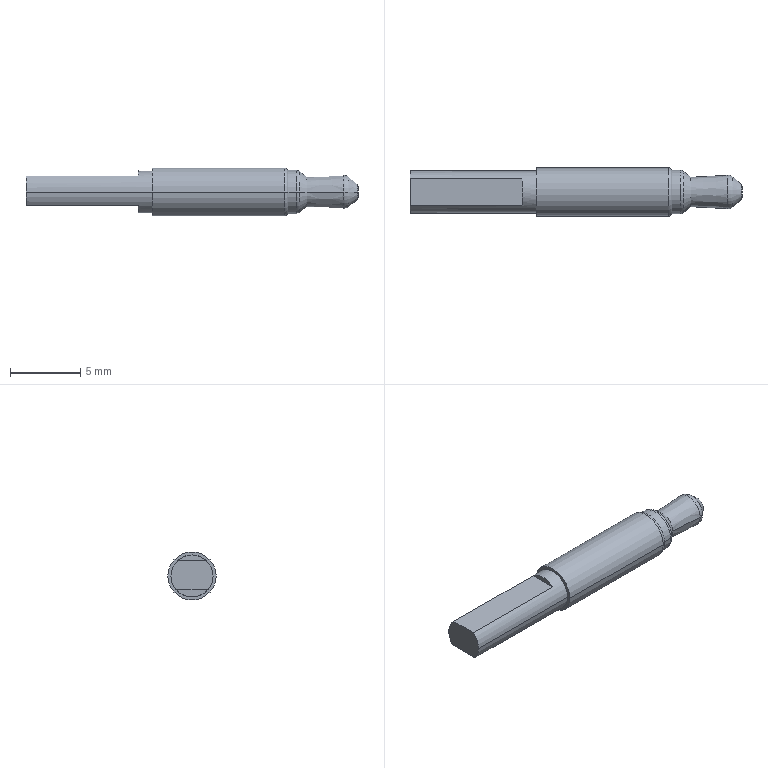Part | NX | 1 solid | 27 faces | box 23.7 x 3.45 x 3.45 mm | volume 165.514 mm3 | torus 8 | plane 7 | cylinder 6 | cone 6 | commonest cylinder face diameters 3 x2 3.1 x2 3.45 x2
STEP:
#1=CARTESIAN_POINT('',(12.641,-1.55,0.));
#2=VERTEX_POINT('',#1);
#3=CARTESIAN_POINT('',(12.641,1.55,0.));
#4=VERTEX_POINT('',#3);
#5=CARTESIAN_POINT('',(12.641,0.,0.));
#6=DIRECTION('',(1.,0.,0.));
#7=DIRECTION('',(0.,-1.,0.));
#8=AXIS2_PLACEMENT_3D('',#5,#6,#7);
#9=CIRCLE('',#8,1.55);
#10=EDGE_CURVE('',#2,#4,#9,.T.);
#11=ORIENTED_EDGE('',*,*,#10,.F.);
#12=CARTESIAN_POINT('',(12.,-1.55,0.));
#13=VERTEX_POINT('',#12);
#14=CARTESIAN_POINT('',(-0.85,-1.55,0.));
#15=DIRECTION('',(1.,0.,0.));
#16=VECTOR('',#15,1000.);
#17=LINE('',#14,#16);
#18=EDGE_CURVE('',#2,#13,#17,.F.);
#19=ORIENTED_EDGE('',*,*,#18,.T.);
#20=CARTESIAN_POINT('',(12.,1.55,0.));
#21=VERTEX_POINT('',#20);
#22=CARTESIAN_POINT('',(12.,0.,0.));
#23=DIRECTION('',(1.,0.,0.));
#24=DIRECTION('',(0.,1.,0.));
#25=AXIS2_PLACEMENT_3D('',#22,#23,#24);
#26=CIRCLE('',#25,1.55);
#27=EDGE_CURVE('',#13,#21,#26,.T.);
#28=ORIENTED_EDGE('',*,*,#27,.T.);
#29=CARTESIAN_POINT('',(-0.85,1.55,0.));
#30=DIRECTION('',(1.,0.,0.));
#31=VECTOR('',#30,1000.);
#32=LINE('',#29,#31);
#33=EDGE_CURVE('',#4,#21,#32,.F.);
#34=ORIENTED_EDGE('',*,*,#33,.F.);
#35=EDGE_LOOP('',(#11,#19,#28,#34));
#36=FACE_BOUND('',#35,.T.);
#37=CARTESIAN_POINT('',(-0.85,0.,0.));
#38=DIRECTION('',(1.,0.,0.));
#39=DIRECTION('',(0.,-1.,0.));
#40=AXIS2_PLACEMENT_3D('',#37,#38,#39);
#41=CYLINDRICAL_SURFACE('',#40,1.55);
#42=ADVANCED_FACE('',(#36),#41,.T.);
#43=CARTESIAN_POINT('',(13.35,1.05,0.));
#44=VERTEX_POINT('',#43);
#45=CARTESIAN_POINT('',(13.35,-1.05,0.));
#46=VERTEX_POINT('',#45);
#47=CARTESIAN_POINT('',(13.35,0.,0.));
#48=DIRECTION('',(1.,0.,0.));
#49=DIRECTION('',(0.,0.,-1.));
#50=AXIS2_PLACEMENT_3D('',#47,#48,#49);
#51=CIRCLE('',#50,1.05);
#52=EDGE_CURVE('',#44,#46,#51,.T.);
#53=ORIENTED_EDGE('',*,*,#52,.F.);
#54=CARTESIAN_POINT('',(12.833,1.48,0.));
#55=VERTEX_POINT('',#54);
#56=CARTESIAN_POINT('',(13.05,1.3,0.));
#57=DIRECTION('',(-0.7682,0.6402,0.));
#58=VECTOR('',#57,1000.);
#59=LINE('',#56,#58);
#60=EDGE_CURVE('',#44,#55,#59,.T.);
#61=ORIENTED_EDGE('',*,*,#60,.T.);
#62=CARTESIAN_POINT('',(12.833,-1.48,0.));
#63=VERTEX_POINT('',#62);
#64=CARTESIAN_POINT('',(12.833,0.,0.));
#65=DIRECTION('',(1.,0.,0.));
#66=DIRECTION('',(0.,-1.,0.));
#67=AXIS2_PLACEMENT_3D('',#64,#65,#66);
#68=CIRCLE('',#67,1.48);
#69=EDGE_CURVE('',#55,#63,#68,.T.);
#70=ORIENTED_EDGE('',*,*,#69,.T.);
#71=CARTESIAN_POINT('',(13.05,-1.3,0.));
#72=DIRECTION('',(-0.7682,-0.6402,0.));
#73=VECTOR('',#72,1000.);
#74=LINE('',#71,#73);
#75=EDGE_CURVE('',#46,#63,#74,.T.);
#76=ORIENTED_EDGE('',*,*,#75,.F.);
#77=EDGE_LOOP('',(#53,#61,#70,#76));
#78=FACE_BOUND('',#77,.T.);
#79=CARTESIAN_POINT('',(13.05,0.,0.));
#80=DIRECTION('',(-1.,0.,0.));
#81=DIRECTION('',(0.,1.,0.));
#82=AXIS2_PLACEMENT_3D('',#79,#80,#81);
#83=CONICAL_SURFACE('',#82,1.3,0.6947);
#84=ADVANCED_FACE('',(#78),#83,.T.);
#85=CARTESIAN_POINT('',(16.932,-0.5598,0.));
#86=VERTEX_POINT('',#85);
#87=CARTESIAN_POINT('',(16.932,0.5598,0.));
#88=VERTEX_POINT('',#87);
#89=CARTESIAN_POINT('',(16.932,0.,0.));
#90=DIRECTION('',(-1.,0.,0.));
#91=DIRECTION('',(0.,-1.,0.));
#92=AXIS2_PLACEMENT_3D('',#89,#90,#91);
#93=CIRCLE('',#92,0.5598);
#94=EDGE_CURVE('',#86,#88,#93,.T.);
#95=ORIENTED_EDGE('',*,*,#94,.T.);
#96=CARTESIAN_POINT('',(16.353,1.066,0.));
#97=VERTEX_POINT('',#96);
#98=CARTESIAN_POINT('',(16.596,0.8531,0.));
#99=DIRECTION('',(-0.7526,0.6585,0.));
#100=VECTOR('',#99,1000.);
#101=LINE('',#98,#100);
#102=EDGE_CURVE('',#88,#97,#101,.T.);
#103=ORIENTED_EDGE('',*,*,#102,.T.);
#104=CARTESIAN_POINT('',(16.353,-1.066,0.));
#105=VERTEX_POINT('',#104);
#106=CARTESIAN_POINT('',(16.353,0.,0.));
#107=DIRECTION('',(-1.,0.,0.));
#108=DIRECTION('',(0.,1.,0.));
#109=AXIS2_PLACEMENT_3D('',#106,#107,#108);
#110=CIRCLE('',#109,1.066);
#111=EDGE_CURVE('',#105,#97,#110,.T.);
#112=ORIENTED_EDGE('',*,*,#111,.F.);
#113=CARTESIAN_POINT('',(16.596,-0.8531,0.));
#114=DIRECTION('',(-0.7526,-0.6585,0.));
#115=VECTOR('',#114,1000.);
#116=LINE('',#113,#115);
#117=EDGE_CURVE('',#86,#105,#116,.T.);
#118=ORIENTED_EDGE('',*,*,#117,.F.);
#119=EDGE_LOOP('',(#95,#103,#112,#118));
#120=FACE_BOUND('',#119,.T.);
#121=CARTESIAN_POINT('',(16.596,0.,0.));
#122=DIRECTION('',(-1.,0.,0.));
#123=DIRECTION('',(0.,1.,0.));
#124=AXIS2_PLACEMENT_3D('',#121,#122,#123);
#125=CONICAL_SURFACE('',#124,0.8531,0.7188);
#126=ADVANCED_FACE('',(#120),#125,.T.);
#127=CARTESIAN_POINT('',(17.,-0.4092,0.));
#128=VERTEX_POINT('',#127);
#129=CARTESIAN_POINT('',(17.,0.4092,0.));
#130=VERTEX_POINT('',#129);
#131=CARTESIAN_POINT('',(17.,0.,0.));
#132=DIRECTION('',(1.,0.,0.));
#133=DIRECTION('',(0.,-1.,0.));
#134=AXIS2_PLACEMENT_3D('',#131,#132,#133);
#135=CIRCLE('',#134,0.4092);
#136=EDGE_CURVE('',#128,#130,#135,.T.);
#137=ORIENTED_EDGE('',*,*,#136,.T.);
#138=CARTESIAN_POINT('',(17.,0.,0.));
#139=DIRECTION('',(1.,0.,0.));
#140=DIRECTION('',(0.,-1.,0.));
#141=AXIS2_PLACEMENT_3D('',#138,#139,#140);
#142=CIRCLE('',#141,0.4092);
#143=EDGE_CURVE('',#130,#128,#142,.T.);
#144=ORIENTED_EDGE('',*,*,#143,.T.);
#145=EDGE_LOOP('',(#137,#144));
#146=FACE_BOUND('',#145,.T.);
#147=CARTESIAN_POINT('',(17.,0.,0.));
#148=DIRECTION('',(1.,0.,0.));
#149=DIRECTION('',(0.,1.,0.));
#150=AXIS2_PLACEMENT_3D('',#147,#148,#149);
#151=PLANE('',#150);
#152=ADVANCED_FACE('',(#146),#151,.T.);
#153=CARTESIAN_POINT('',(11.727,-1.725,0.));
#154=VERTEX_POINT('',#153);
#155=CARTESIAN_POINT('',(11.727,1.725,0.));
#156=VERTEX_POINT('',#155);
#157=CARTESIAN_POINT('',(11.727,0.,0.));
#158=DIRECTION('',(1.,0.,0.));
#159=DIRECTION('',(0.,-1.,0.));
#160=AXIS2_PLACEMENT_3D('',#157,#158,#159);
#161=CIRCLE('',#160,1.725);
#162=EDGE_CURVE('',#154,#156,#161,.T.);
#163=ORIENTED_EDGE('',*,*,#162,.T.);
#164=CARTESIAN_POINT('',(11.727,1.425,0.));
#165=DIRECTION('',(0.,0.,1.));
#166=DIRECTION('',(-1.,0.,0.));
#167=AXIS2_PLACEMENT_3D('',#164,#165,#166);
#168=CIRCLE('',#167,0.3);
#169=EDGE_CURVE('',#21,#156,#168,.T.);
#170=ORIENTED_EDGE('',*,*,#169,.F.);
#171=ORIENTED_EDGE('',*,*,#27,.F.);
#172=CARTESIAN_POINT('',(11.727,-1.425,0.));
#173=DIRECTION('',(0.,0.,-1.));
#174=DIRECTION('',(-1.,0.,0.));
#175=AXIS2_PLACEMENT_3D('',#172,#173,#174);
#176=CIRCLE('',#175,0.3);
#177=EDGE_CURVE('',#13,#154,#176,.T.);
#178=ORIENTED_EDGE('',*,*,#177,.T.);
#179=EDGE_LOOP('',(#163,#170,#171,#178));
#180=FACE_BOUND('',#179,.T.);
#181=CARTESIAN_POINT('',(11.727,0.,0.));
#182=DIRECTION('',(1.,0.,0.));
#183=DIRECTION('',(0.,-1.,0.));
#184=AXIS2_PLACEMENT_3D('',#181,#182,#183);
#185=TOROIDAL_SURFACE('',#184,1.425,0.3);
#186=ADVANCED_FACE('',(#180),#185,.T.);
#187=CARTESIAN_POINT('',(15.997,-1.189,0.));
#188=VERTEX_POINT('',#187);
#189=CARTESIAN_POINT('',(15.997,1.189,0.));
#190=VERTEX_POINT('',#189);
#191=CARTESIAN_POINT('',(15.997,0.,0.));
#192=DIRECTION('',(-1.,0.,0.));
#193=DIRECTION('',(0.,1.,0.));
#194=AXIS2_PLACEMENT_3D('',#191,#192,#193);
#195=CIRCLE('',#194,1.189);
#196=EDGE_CURVE('',#188,#190,#195,.T.);
#197=ORIENTED_EDGE('',*,*,#196,.F.);
#198=CARTESIAN_POINT('',(16.024,-0.69,0.));
#199=DIRECTION('',(0.,0.,1.));
#200=DIRECTION('',(-1.,0.,0.));
#201=AXIS2_PLACEMENT_3D('',#198,#199,#200);
#202=CIRCLE('',#201,0.5);
#203=EDGE_CURVE('',#188,#105,#202,.T.);
#204=ORIENTED_EDGE('',*,*,#203,.T.);
#205=ORIENTED_EDGE('',*,*,#111,.T.);
#206=CARTESIAN_POINT('',(16.024,0.69,0.));
#207=DIRECTION('',(0.,0.,-1.));
#208=DIRECTION('',(-1.,0.,0.));
#209=AXIS2_PLACEMENT_3D('',#206,#207,#208);
#210=CIRCLE('',#209,0.5);
#211=EDGE_CURVE('',#190,#97,#210,.T.);
#212=ORIENTED_EDGE('',*,*,#211,.F.);
#213=EDGE_LOOP('',(#197,#204,#205,#212));
#214=FACE_BOUND('',#213,.T.);
#215=CARTESIAN_POINT('',(16.024,0.,0.));
#216=DIRECTION('',(-1.,0.,0.));
#217=DIRECTION('',(0.,1.,0.));
#218=AXIS2_PLACEMENT_3D('',#215,#216,#217);
#219=TOROIDAL_SURFACE('',#218,0.69,0.5);
#220=ADVANCED_FACE('',(#214),#219,.T.);
#221=CARTESIAN_POINT('',(2.3,1.725,0.));
#222=VERTEX_POINT('',#221);
#223=CARTESIAN_POINT('',(2.3,-1.725,0.));
#224=VERTEX_POINT('',#223);
#225=CARTESIAN_POINT('',(2.3,0.,0.));
#226=DIRECTION('',(1.,0.,0.));
#227=DIRECTION('',(0.,-1.,0.));
#228=AXIS2_PLACEMENT_3D('',#225,#226,#227);
#229=CIRCLE('',#228,1.725);
#230=EDGE_CURVE('',#222,#224,#229,.T.);
#231=ORIENTED_EDGE('',*,*,#230,.T.);
#232=CARTESIAN_POINT('',(0.,-1.725,0.));
#233=DIRECTION('',(1.,0.,0.));
#234=VECTOR('',#233,1000.);
#235=LINE('',#232,#234);
#236=EDGE_CURVE('',#154,#224,#235,.F.);
#237=ORIENTED_EDGE('',*,*,#236,.F.);
#238=CARTESIAN_POINT('',(11.727,0.,0.));
#239=DIRECTION('',(1.,0.,0.));
#240=DIRECTION('',(0.,-1.,0.));
#241=AXIS2_PLACEMENT_3D('',#238,#239,#240);
#242=CIRCLE('',#241,1.725);
#243=EDGE_CURVE('',#156,#154,#242,.T.);
#244=ORIENTED_EDGE('',*,*,#243,.F.);
#245=CARTESIAN_POINT('',(0.,1.725,0.));
#246=DIRECTION('',(1.,0.,0.));
#247=VECTOR('',#246,1000.);
#248=LINE('',#245,#247);
#249=EDGE_CURVE('',#156,#222,#248,.F.);
#250=ORIENTED_EDGE('',*,*,#249,.T.);
#251=EDGE_LOOP('',(#231,#237,#244,#250));
#252=FACE_BOUND('',#251,.T.);
#253=CARTESIAN_POINT('',(0.,0.,0.));
#254=DIRECTION('',(1.,0.,0.));
#255=DIRECTION('',(0.,-1.,0.));
#256=AXIS2_PLACEMENT_3D('',#253,#254,#255);
#257=CYLINDRICAL_SURFACE('',#256,1.725);
#258=ADVANCED_FACE('',(#252),#257,.T.);
#259=ORIENTED_EDGE('',*,*,#52,.T.);
#260=CARTESIAN_POINT('',(14.734,-1.123,0.));
#261=DIRECTION('',(0.9986,-0.05256,0.));
#262=VECTOR('',#261,1000.);
#263=LINE('',#260,#262);
#264=EDGE_CURVE('',#188,#46,#263,.F.);
#265=ORIENTED_EDGE('',*,*,#264,.F.);
#266=ORIENTED_EDGE('',*,*,#196,.T.);
#267=CARTESIAN_POINT('',(14.734,1.123,0.));
#268=DIRECTION('',(0.9986,0.05256,0.));
#269=VECTOR('',#268,1000.);
#270=LINE('',#267,#269);
#271=EDGE_CURVE('',#190,#44,#270,.F.);
#272=ORIENTED_EDGE('',*,*,#271,.T.);
#273=EDGE_LOOP('',(#259,#265,#266,#272));
#274=FACE_BOUND('',#273,.T.);
#275=CARTESIAN_POINT('',(14.734,0.,0.));
#276=DIRECTION('',(1.,0.,0.));
#277=DIRECTION('',(0.,-1.,0.));
#278=AXIS2_PLACEMENT_3D('',#275,#276,#277);
#279=CONICAL_SURFACE('',#278,1.123,0.05258);
#280=ADVANCED_FACE('',(#274),#279,.T.);
#281=CARTESIAN_POINT('',(12.833,0.,0.));
#282=DIRECTION('',(1.,0.,0.));
#283=DIRECTION('',(0.,-1.,0.));
#284=AXIS2_PLACEMENT_3D('',#281,#282,#283);
#285=CIRCLE('',#284,1.48);
#286=EDGE_CURVE('',#63,#55,#285,.T.);
#287=ORIENTED_EDGE('',*,*,#286,.F.);
#288=CARTESIAN_POINT('',(12.641,-1.25,0.));
#289=DIRECTION('',(0.,0.,-1.));
#290=DIRECTION('',(-1.,0.,0.));
#291=AXIS2_PLACEMENT_3D('',#288,#289,#290);
#292=CIRCLE('',#291,0.3);
#293=EDGE_CURVE('',#2,#63,#292,.F.);
#294=ORIENTED_EDGE('',*,*,#293,.F.);
#295=ORIENTED_EDGE('',*,*,#10,.T.);
#296=CARTESIAN_POINT('',(12.641,1.25,0.));
#297=DIRECTION('',(0.,0.,1.));
#298=DIRECTION('',(-1.,0.,0.));
#299=AXIS2_PLACEMENT_3D('',#296,#297,#298);
#300=CIRCLE('',#299,0.3);
#301=EDGE_CURVE('',#4,#55,#300,.F.);
#302=ORIENTED_EDGE('',*,*,#301,.T.);
#303=EDGE_LOOP('',(#287,#294,#295,#302));
#304=FACE_BOUND('',#303,.T.);
#305=CARTESIAN_POINT('',(12.641,0.,0.));
#306=DIRECTION('',(1.,0.,0.));
#307=DIRECTION('',(0.,-1.,0.));
#308=AXIS2_PLACEMENT_3D('',#305,#306,#307);
#309=TOROIDAL_SURFACE('',#308,1.25,0.3);
#310=ADVANCED_FACE('',(#304),#309,.T.);
#311=ORIENTED_EDGE('',*,*,#136,.F.);
#312=CARTESIAN_POINT('',(16.8,-0.4092,0.));
#313=DIRECTION('',(0.,0.,-1.));
#314=DIRECTION('',(-1.,0.,0.));
#315=AXIS2_PLACEMENT_3D('',#312,#313,#314);
#316=CIRCLE('',#315,0.2);
#317=EDGE_CURVE('',#86,#128,#316,.F.);
#318=ORIENTED_EDGE('',*,*,#317,.F.);
#319=CARTESIAN_POINT('',(16.932,0.,0.));
#320=DIRECTION('',(-1.,0.,0.));
#321=DIRECTION('',(0.,-1.,0.));
#322=AXIS2_PLACEMENT_3D('',#319,#320,#321);
#323=CIRCLE('',#322,0.5598);
#324=EDGE_CURVE('',#88,#86,#323,.T.);
#325=ORIENTED_EDGE('',*,*,#324,.F.);
#326=CARTESIAN_POINT('',(16.8,0.4092,0.));
#327=DIRECTION('',(0.,0.,1.));
#328=DIRECTION('',(-1.,0.,0.));
#329=AXIS2_PLACEMENT_3D('',#326,#327,#328);
#330=CIRCLE('',#329,0.2);
#331=EDGE_CURVE('',#88,#130,#330,.F.);
#332=ORIENTED_EDGE('',*,*,#331,.T.);
#333=EDGE_LOOP('',(#311,#318,#325,#332));
#334=FACE_BOUND('',#333,.T.);
#335=CARTESIAN_POINT('',(16.8,0.,0.));
#336=DIRECTION('',(1.,0.,0.));
#337=DIRECTION('',(0.,-1.,0.));
#338=AXIS2_PLACEMENT_3D('',#335,#336,#337);
#339=TOROIDAL_SURFACE('',#338,0.4092,0.2);
#340=ADVANCED_FACE('',(#334),#339,.T.);
#341=ORIENTED_EDGE('',*,*,#230,.F.);
#342=CARTESIAN_POINT('',(2.3,0.,0.));
#343=DIRECTION('',(1.,0.,0.));
#344=DIRECTION('',(0.,-1.,0.));
#345=AXIS2_PLACEMENT_3D('',#342,#343,#344);
#346=CIRCLE('',#345,1.725);
#347=EDGE_CURVE('',#224,#222,#346,.T.);
#348=ORIENTED_EDGE('',*,*,#347,.F.);
#349=EDGE_LOOP('',(#341,#348));
#350=FACE_BOUND('',#349,.T.);
#351=CARTESIAN_POINT('',(2.3,-1.5,0.));
#352=VERTEX_POINT('',#351);
#353=CARTESIAN_POINT('',(2.3,1.5,0.));
#354=VERTEX_POINT('',#353);
#355=CARTESIAN_POINT('',(2.3,0.,0.));
#356=DIRECTION('',(-1.,0.,0.));
#357=DIRECTION('',(0.,-1.,0.));
#358=AXIS2_PLACEMENT_3D('',#355,#356,#357);
#359=CIRCLE('',#358,1.5);
#360=EDGE_CURVE('',#352,#354,#359,.T.);
#361=ORIENTED_EDGE('',*,*,#360,.F.);
#362=CARTESIAN_POINT('',(2.3,0.,0.));
#363=DIRECTION('',(-1.,0.,0.));
#364=DIRECTION('',(0.,-1.,0.));
#365=AXIS2_PLACEMENT_3D('',#362,#363,#364);
#366=CIRCLE('',#365,1.5);
#367=EDGE_CURVE('',#354,#352,#366,.T.);
#368=ORIENTED_EDGE('',*,*,#367,.F.);
#369=EDGE_LOOP('',(#361,#368));
#370=FACE_BOUND('',#369,.T.);
#371=CARTESIAN_POINT('',(2.3,-28.452,3.6));
#372=DIRECTION('',(1.,0.,0.));
#373=DIRECTION('',(0.,0.,1.));
#374=AXIS2_PLACEMENT_3D('',#371,#372,#373);
#375=PLANE('',#374);
#376=ADVANCED_FACE('',(#350,#370),#375,.F.);
#377=CARTESIAN_POINT('',(-6.7,1.5,0.));
#378=VERTEX_POINT('',#377);
#379=CARTESIAN_POINT('',(-6.7,1.144,-0.97));
#380=VERTEX_POINT('',#379);
#381=CARTESIAN_POINT('',(-6.7,0.,0.));
#382=DIRECTION('',(-1.,0.,0.));
#383=DIRECTION('',(0.,-1.,0.));
#384=AXIS2_PLACEMENT_3D('',#381,#382,#383);
#385=CIRCLE('',#384,1.5);
#386=EDGE_CURVE('',#378,#380,#385,.T.);
#387=ORIENTED_EDGE('',*,*,#386,.F.);
#388=CARTESIAN_POINT('',(2.3,1.5,0.));
#389=DIRECTION('',(-1.,0.,0.));
#390=VECTOR('',#389,1000.);
#391=LINE('',#388,#390);
#392=EDGE_CURVE('',#354,#378,#391,.T.);
#393=ORIENTED_EDGE('',*,*,#392,.F.);
#394=ORIENTED_EDGE('',*,*,#367,.T.);
#395=CARTESIAN_POINT('',(-6.7,-1.5,0.));
#396=VERTEX_POINT('',#395);
#397=CARTESIAN_POINT('',(2.3,-1.5,0.));
#398=DIRECTION('',(-1.,0.,0.));
#399=VECTOR('',#398,1000.);
#400=LINE('',#397,#399);
#401=EDGE_CURVE('',#352,#396,#400,.T.);
#402=ORIENTED_EDGE('',*,*,#401,.T.);
#403=CARTESIAN_POINT('',(-6.7,-1.144,-0.97));
#404=VERTEX_POINT('',#403);
#405=CARTESIAN_POINT('',(-6.7,0.,0.));
#406=DIRECTION('',(-1.,0.,0.));
#407=DIRECTION('',(0.,-1.,0.));
#408=AXIS2_PLACEMENT_3D('',#405,#406,#407);
#409=CIRCLE('',#408,1.5);
#410=EDGE_CURVE('',#404,#396,#409,.T.);
#411=ORIENTED_EDGE('',*,*,#410,.F.);
#412=CARTESIAN_POINT('',(1.3,-1.144,-0.97));
#413=VERTEX_POINT('',#412);
#414=CARTESIAN_POINT('',(2.3,-1.144,-0.97));
#415=DIRECTION('',(-1.,0.,0.));
#416=VECTOR('',#415,1000.);
#417=LINE('',#414,#416);
#418=EDGE_CURVE('',#404,#413,#417,.F.);
#419=ORIENTED_EDGE('',*,*,#418,.T.);
#420=CARTESIAN_POINT('',(1.3,1.144,-0.97));
#421=VERTEX_POINT('',#420);
#422=CARTESIAN_POINT('',(1.3,0.,0.));
#423=DIRECTION('',(-1.,0.,0.));
#424=DIRECTION('',(0.,-1.,0.));
#425=AXIS2_PLACEMENT_3D('',#422,#423,#424);
#426=CIRCLE('',#425,1.5);
#427=EDGE_CURVE('',#421,#413,#426,.T.);
#428=ORIENTED_EDGE('',*,*,#427,.F.);
#429=CARTESIAN_POINT('',(2.3,1.144,-0.97));
#430=DIRECTION('',(-1.,0.,0.));
#431=VECTOR('',#430,1000.);
#432=LINE('',#429,#431);
#433=EDGE_CURVE('',#380,#421,#432,.F.);
#434=ORIENTED_EDGE('',*,*,#433,.F.);
#435=EDGE_LOOP('',(#387,#393,#394,#402,#411,#419,#428,#434));
#436=FACE_BOUND('',#435,.T.);
#437=CARTESIAN_POINT('',(2.3,0.,0.));
#438=DIRECTION('',(-1.,0.,0.));
#439=DIRECTION('',(0.,-1.,0.));
#440=AXIS2_PLACEMENT_3D('',#437,#438,#439);
#441=CYLINDRICAL_SURFACE('',#440,1.5);
#442=ADVANCED_FACE('',(#436),#441,.T.);
#443=ORIENTED_EDGE('',*,*,#386,.T.);
#444=CARTESIAN_POINT('',(-6.7,0.,-0.97));
#445=DIRECTION('',(0.,1.,0.));
#446=VECTOR('',#445,1000.);
#447=LINE('',#444,#446);
#448=EDGE_CURVE('',#404,#380,#447,.T.);
#449=ORIENTED_EDGE('',*,*,#448,.F.);
#450=ORIENTED_EDGE('',*,*,#410,.T.);
#451=CARTESIAN_POINT('',(-6.7,-0.9864,1.13));
#452=VERTEX_POINT('',#451);
#453=CARTESIAN_POINT('',(-6.7,0.,0.));
#454=DIRECTION('',(-1.,0.,0.));
#455=DIRECTION('',(0.,-1.,0.));
#456=AXIS2_PLACEMENT_3D('',#453,#454,#455);
#457=CIRCLE('',#456,1.5);
#458=EDGE_CURVE('',#396,#452,#457,.T.);
#459=ORIENTED_EDGE('',*,*,#458,.T.);
#460=CARTESIAN_POINT('',(-6.7,0.9864,1.13));
#461=VERTEX_POINT('',#460);
#462=CARTESIAN_POINT('',(-6.7,0.,1.13));
#463=DIRECTION('',(0.,-1.,0.));
#464=VECTOR('',#463,1000.);
#465=LINE('',#462,#464);
#466=EDGE_CURVE('',#461,#452,#465,.T.);
#467=ORIENTED_EDGE('',*,*,#466,.F.);
#468=CARTESIAN_POINT('',(-6.7,0.,0.));
#469=DIRECTION('',(-1.,0.,0.));
#470=DIRECTION('',(0.,-1.,0.));
#471=AXIS2_PLACEMENT_3D('',#468,#469,#470);
#472=CIRCLE('',#471,1.5);
#473=EDGE_CURVE('',#461,#378,#472,.T.);
#474=ORIENTED_EDGE('',*,*,#473,.T.);
#475=EDGE_LOOP('',(#443,#449,#450,#459,#467,#474));
#476=FACE_BOUND('',#475,.T.);
#477=CARTESIAN_POINT('',(-6.7,0.6142,-0.2899));
#478=DIRECTION('',(-1.,0.,0.));
#479=DIRECTION('',(0.,0.,1.));
#480=AXIS2_PLACEMENT_3D('',#477,#478,#479);
#481=PLANE('',#480);
#482=ADVANCED_FACE('',(#476),#481,.T.);
#483=ORIENTED_EDGE('',*,*,#427,.T.);
#484=CARTESIAN_POINT('',(1.3,-1.5,-0.97));
#485=DIRECTION('',(0.,1.,0.));
#486=VECTOR('',#485,1000.);
#487=LINE('',#484,#486);
#488=EDGE_CURVE('',#413,#421,#487,.T.);
#489=ORIENTED_EDGE('',*,*,#488,.T.);
#490=EDGE_LOOP('',(#483,#489));
#491=FACE_BOUND('',#490,.T.);
#492=CARTESIAN_POINT('',(1.3,1.5,-2.47));
#493=DIRECTION('',(1.,0.,0.));
#494=DIRECTION('',(0.,0.,1.));
#495=AXIS2_PLACEMENT_3D('',#492,#493,#494);
#496=PLANE('',#495);
#497=ADVANCED_FACE('',(#491),#496,.F.);
#498=ORIENTED_EDGE('',*,*,#418,.F.);
#499=ORIENTED_EDGE('',*,*,#448,.T.);
#500=ORIENTED_EDGE('',*,*,#433,.T.);
#501=ORIENTED_EDGE('',*,*,#488,.F.);
#502=EDGE_LOOP('',(#498,#499,#500,#501));
#503=FACE_BOUND('',#502,.T.);
#504=CARTESIAN_POINT('',(-3.393,-0.2163,-0.97));
#505=DIRECTION('',(0.,0.,-1.));
#506=DIRECTION('',(0.,-1.,0.));
#507=AXIS2_PLACEMENT_3D('',#504,#505,#506);
#508=PLANE('',#507);
#509=ADVANCED_FACE('',(#503),#508,.T.);
#510=CARTESIAN_POINT('',(1.3,-0.9864,1.13));
#511=VERTEX_POINT('',#510);
#512=CARTESIAN_POINT('',(1.3,0.9864,1.13));
#513=VERTEX_POINT('',#512);
#514=CARTESIAN_POINT('',(1.3,0.,0.));
#515=DIRECTION('',(-1.,0.,0.));
#516=DIRECTION('',(0.,-1.,0.));
#517=AXIS2_PLACEMENT_3D('',#514,#515,#516);
#518=CIRCLE('',#517,1.5);
#519=EDGE_CURVE('',#511,#513,#518,.T.);
#520=ORIENTED_EDGE('',*,*,#519,.T.);
#521=CARTESIAN_POINT('',(1.3,-5.456,1.13));
#522=DIRECTION('',(0.,1.,0.));
#523=VECTOR('',#522,1000.);
#524=LINE('',#521,#523);
#525=EDGE_CURVE('',#511,#513,#524,.T.);
#526=ORIENTED_EDGE('',*,*,#525,.F.);
#527=EDGE_LOOP('',(#520,#526));
#528=FACE_BOUND('',#527,.T.);
#529=CARTESIAN_POINT('',(1.3,-5.456,3.53));
#530=DIRECTION('',(1.,0.,0.));
#531=DIRECTION('',(0.,1.,0.));
#532=AXIS2_PLACEMENT_3D('',#529,#530,#531);
#533=PLANE('',#532);
#534=ADVANCED_FACE('',(#528),#533,.F.);
#535=CARTESIAN_POINT('',(2.3,0.9864,1.13));
#536=DIRECTION('',(-1.,0.,0.));
#537=VECTOR('',#536,1000.);
#538=LINE('',#535,#537);
#539=EDGE_CURVE('',#513,#461,#538,.T.);
#540=ORIENTED_EDGE('',*,*,#539,.T.);
#541=ORIENTED_EDGE('',*,*,#466,.T.);
#542=CARTESIAN_POINT('',(2.3,-0.9864,1.13));
#543=DIRECTION('',(-1.,0.,0.));
#544=VECTOR('',#543,1000.);
#545=LINE('',#542,#544);
#546=EDGE_CURVE('',#511,#452,#545,.T.);
#547=ORIENTED_EDGE('',*,*,#546,.F.);
#548=ORIENTED_EDGE('',*,*,#525,.T.);
#549=EDGE_LOOP('',(#540,#541,#547,#548));
#550=FACE_BOUND('',#549,.T.);
#551=CARTESIAN_POINT('',(-5.112,-0.01314,1.13));
#552=DIRECTION('',(0.,0.,1.));
#553=DIRECTION('',(1.,0.,0.));
#554=AXIS2_PLACEMENT_3D('',#551,#552,#553);
#555=PLANE('',#554);
#556=ADVANCED_FACE('',(#550),#555,.T.);
#557=ORIENTED_EDGE('',*,*,#102,.F.);
#558=ORIENTED_EDGE('',*,*,#324,.T.);
#559=ORIENTED_EDGE('',*,*,#117,.T.);
#560=CARTESIAN_POINT('',(16.353,0.,0.));
#561=DIRECTION('',(-1.,0.,0.));
#562=DIRECTION('',(0.,1.,0.));
#563=AXIS2_PLACEMENT_3D('',#560,#561,#562);
#564=CIRCLE('',#563,1.066);
#565=EDGE_CURVE('',#97,#105,#564,.T.);
#566=ORIENTED_EDGE('',*,*,#565,.F.);
#567=EDGE_LOOP('',(#557,#558,#559,#566));
#568=FACE_BOUND('',#567,.T.);
#569=CARTESIAN_POINT('',(16.596,0.,0.));
#570=DIRECTION('',(-1.,0.,0.));
#571=DIRECTION('',(0.,1.,0.));
#572=AXIS2_PLACEMENT_3D('',#569,#570,#571);
#573=CONICAL_SURFACE('',#572,0.8531,0.7188);
#574=ADVANCED_FACE('',(#568),#573,.T.);
#575=ORIENTED_EDGE('',*,*,#360,.T.);
#576=ORIENTED_EDGE('',*,*,#392,.T.);
#577=ORIENTED_EDGE('',*,*,#473,.F.);
#578=ORIENTED_EDGE('',*,*,#539,.F.);
#579=ORIENTED_EDGE('',*,*,#519,.F.);
#580=ORIENTED_EDGE('',*,*,#546,.T.);
#581=ORIENTED_EDGE('',*,*,#458,.F.);
#582=ORIENTED_EDGE('',*,*,#401,.F.);
#583=EDGE_LOOP('',(#575,#576,#577,#578,#579,#580,#581,#582));
#584=FACE_BOUND('',#583,.T.);
#585=CARTESIAN_POINT('',(2.3,0.,0.));
#586=DIRECTION('',(-1.,0.,0.));
#587=DIRECTION('',(0.,-1.,0.));
#588=AXIS2_PLACEMENT_3D('',#585,#586,#587);
#589=CYLINDRICAL_SURFACE('',#588,1.5);
#590=ADVANCED_FACE('',(#584),#589,.T.);
#591=ORIENTED_EDGE('',*,*,#264,.T.);
#592=CARTESIAN_POINT('',(13.35,0.,0.));
#593=DIRECTION('',(1.,0.,0.));
#594=DIRECTION('',(0.,0.,-1.));
#595=AXIS2_PLACEMENT_3D('',#592,#593,#594);
#596=CIRCLE('',#595,1.05);
#597=EDGE_CURVE('',#46,#44,#596,.T.);
#598=ORIENTED_EDGE('',*,*,#597,.T.);
#599=ORIENTED_EDGE('',*,*,#271,.F.);
#600=CARTESIAN_POINT('',(15.997,0.,0.));
#601=DIRECTION('',(-1.,0.,0.));
#602=DIRECTION('',(0.,1.,0.));
#603=AXIS2_PLACEMENT_3D('',#600,#601,#602);
#604=CIRCLE('',#603,1.189);
#605=EDGE_CURVE('',#190,#188,#604,.T.);
#606=ORIENTED_EDGE('',*,*,#605,.T.);
#607=EDGE_LOOP('',(#591,#598,#599,#606));
#608=FACE_BOUND('',#607,.T.);
#609=CARTESIAN_POINT('',(14.734,0.,0.));
#610=DIRECTION('',(1.,0.,0.));
#611=DIRECTION('',(0.,-1.,0.));
#612=AXIS2_PLACEMENT_3D('',#609,#610,#611);
#613=CONICAL_SURFACE('',#612,1.123,0.05258);
#614=ADVANCED_FACE('',(#608),#613,.T.);
#615=ORIENTED_EDGE('',*,*,#162,.F.);
#616=ORIENTED_EDGE('',*,*,#236,.T.);
#617=ORIENTED_EDGE('',*,*,#347,.T.);
#618=ORIENTED_EDGE('',*,*,#249,.F.);
#619=EDGE_LOOP('',(#615,#616,#617,#618));
#620=FACE_BOUND('',#619,.T.);
#621=CARTESIAN_POINT('',(0.,0.,0.));
#622=DIRECTION('',(1.,0.,0.));
#623=DIRECTION('',(0.,-1.,0.));
#624=AXIS2_PLACEMENT_3D('',#621,#622,#623);
#625=CYLINDRICAL_SURFACE('',#624,1.725);
#626=ADVANCED_FACE('',(#620),#625,.T.);
#627=ORIENTED_EDGE('',*,*,#286,.T.);
#628=ORIENTED_EDGE('',*,*,#60,.F.);
#629=ORIENTED_EDGE('',*,*,#597,.F.);
#630=ORIENTED_EDGE('',*,*,#75,.T.);
#631=EDGE_LOOP('',(#627,#628,#629,#630));
#632=FACE_BOUND('',#631,.T.);
#633=CARTESIAN_POINT('',(13.05,0.,0.));
#634=DIRECTION('',(-1.,0.,0.));
#635=DIRECTION('',(0.,1.,0.));
#636=AXIS2_PLACEMENT_3D('',#633,#634,#635);
#637=CONICAL_SURFACE('',#636,1.3,0.6947);
#638=ADVANCED_FACE('',(#632),#637,.T.);
#639=CARTESIAN_POINT('',(12.,0.,0.));
#640=DIRECTION('',(1.,0.,0.));
#641=DIRECTION('',(0.,1.,0.));
#642=AXIS2_PLACEMENT_3D('',#639,#640,#641);
#643=CIRCLE('',#642,1.55);
#644=EDGE_CURVE('',#21,#13,#643,.T.);
#645=ORIENTED_EDGE('',*,*,#644,.T.);
#646=ORIENTED_EDGE('',*,*,#18,.F.);
#647=CARTESIAN_POINT('',(12.641,0.,0.));
#648=DIRECTION('',(1.,0.,0.));
#649=DIRECTION('',(0.,-1.,0.));
#650=AXIS2_PLACEMENT_3D('',#647,#648,#649);
#651=CIRCLE('',#650,1.55);
#652=EDGE_CURVE('',#4,#2,#651,.T.);
#653=ORIENTED_EDGE('',*,*,#652,.F.);
#654=ORIENTED_EDGE('',*,*,#33,.T.);
#655=EDGE_LOOP('',(#645,#646,#653,#654));
#656=FACE_BOUND('',#655,.T.);
#657=CARTESIAN_POINT('',(-0.85,0.,0.));
#658=DIRECTION('',(1.,0.,0.));
#659=DIRECTION('',(0.,-1.,0.));
#660=AXIS2_PLACEMENT_3D('',#657,#658,#659);
#661=CYLINDRICAL_SURFACE('',#660,1.55);
#662=ADVANCED_FACE('',(#656),#661,.T.);
#663=ORIENTED_EDGE('',*,*,#211,.T.);
#664=ORIENTED_EDGE('',*,*,#565,.T.);
#665=ORIENTED_EDGE('',*,*,#203,.F.);
#666=ORIENTED_EDGE('',*,*,#605,.F.);
#667=EDGE_LOOP('',(#663,#664,#665,#666));
#668=FACE_BOUND('',#667,.T.);
#669=CARTESIAN_POINT('',(16.024,0.,0.));
#670=DIRECTION('',(-1.,0.,0.));
#671=DIRECTION('',(0.,1.,0.));
#672=AXIS2_PLACEMENT_3D('',#669,#670,#671);
#673=TOROIDAL_SURFACE('',#672,0.69,0.5);
#674=ADVANCED_FACE('',(#668),#673,.T.);
#675=ORIENTED_EDGE('',*,*,#293,.T.);
#676=ORIENTED_EDGE('',*,*,#69,.F.);
#677=ORIENTED_EDGE('',*,*,#301,.F.);
#678=ORIENTED_EDGE('',*,*,#652,.T.);
#679=EDGE_LOOP('',(#675,#676,#677,#678));
#680=FACE_BOUND('',#679,.T.);
#681=CARTESIAN_POINT('',(12.641,0.,0.));
#682=DIRECTION('',(1.,0.,0.));
#683=DIRECTION('',(0.,-1.,0.));
#684=AXIS2_PLACEMENT_3D('',#681,#682,#683);
#685=TOROIDAL_SURFACE('',#684,1.25,0.3);
#686=ADVANCED_FACE('',(#680),#685,.T.);
#687=ORIENTED_EDGE('',*,*,#644,.F.);
#688=ORIENTED_EDGE('',*,*,#169,.T.);
#689=ORIENTED_EDGE('',*,*,#243,.T.);
#690=ORIENTED_EDGE('',*,*,#177,.F.);
#691=EDGE_LOOP('',(#687,#688,#689,#690));
#692=FACE_BOUND('',#691,.T.);
#693=CARTESIAN_POINT('',(11.727,0.,0.));
#694=DIRECTION('',(1.,0.,0.));
#695=DIRECTION('',(0.,-1.,0.));
#696=AXIS2_PLACEMENT_3D('',#693,#694,#695);
#697=TOROIDAL_SURFACE('',#696,1.425,0.3);
#698=ADVANCED_FACE('',(#692),#697,.T.);
#699=ORIENTED_EDGE('',*,*,#94,.F.);
#700=ORIENTED_EDGE('',*,*,#317,.T.);
#701=ORIENTED_EDGE('',*,*,#143,.F.);
#702=ORIENTED_EDGE('',*,*,#331,.F.);
#703=EDGE_LOOP('',(#699,#700,#701,#702));
#704=FACE_BOUND('',#703,.T.);
#705=CARTESIAN_POINT('',(16.8,0.,0.));
#706=DIRECTION('',(1.,0.,0.));
#707=DIRECTION('',(0.,-1.,0.));
#708=AXIS2_PLACEMENT_3D('',#705,#706,#707);
#709=TOROIDAL_SURFACE('',#708,0.4092,0.2);
#710=ADVANCED_FACE('',(#704),#709,.T.);
#711=CLOSED_SHELL('',(#42,#84,#126,#152,#186,#220,#258,#280,#310,#340,#376,#442,#482,#497,#509,#534,#556,#574,#590,#614,#626,#638,#662,#674,#686,#698,#710));
#712=MANIFOLD_SOLID_BREP('',#711);
#713=(LENGTH_UNIT()NAMED_UNIT(*)SI_UNIT(.MILLI.,.METRE.));
#714=UNCERTAINTY_MEASURE_WITH_UNIT(LENGTH_MEASURE(0.00001),#713,'','');
#715=(NAMED_UNIT(*)PLANE_ANGLE_UNIT()SI_UNIT($,.RADIAN.));
#716=(NAMED_UNIT(*)SI_UNIT($,.STERADIAN.)SOLID_ANGLE_UNIT());
#717=(GEOMETRIC_REPRESENTATION_CONTEXT(3)GLOBAL_UNCERTAINTY_ASSIGNED_CONTEXT((#714))GLOBAL_UNIT_ASSIGNED_CONTEXT((#713,#715,#716))REPRESENTATION_CONTEXT('',''));
#718=ADVANCED_BREP_SHAPE_REPRESENTATION('',(#712),#717);